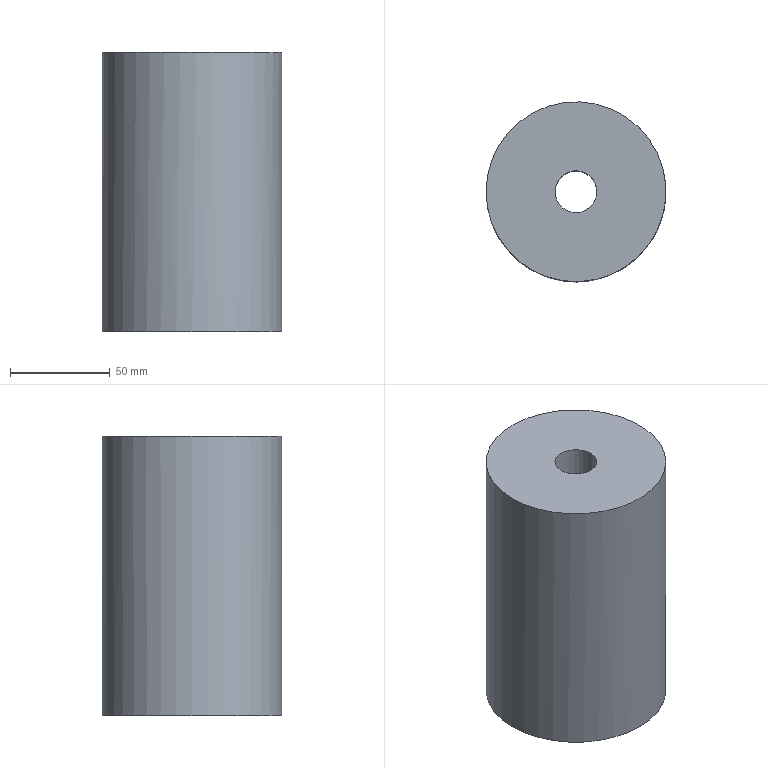Part | NX | features solid 2 | 1 solid | 4 faces | box 90 x 90 x 140 mm | volume 842151 mm3 | cylinder 2 | plane 2 | commonest cylinder face diameters 21 x1 90 x1
STEP:
#1=CARTESIAN_POINT('',(1440.,-535.,-125.));
#2=VERTEX_POINT('',#1);
#3=CARTESIAN_POINT('',(1395.,-535.,-125.));
#4=DIRECTION('',(0.,0.,-1.));
#5=DIRECTION('',(1.,0.,0.));
#6=AXIS2_PLACEMENT_3D('',#3,#4,#5);
#7=CIRCLE('',#6,45.);
#8=EDGE_CURVE('',#2,#2,#7,.F.);
#9=ORIENTED_EDGE('',*,*,#8,.T.);
#10=EDGE_LOOP('',(#9));
#11=FACE_BOUND('',#10,.T.);
#12=CARTESIAN_POINT('',(1350.,-535.,15.));
#13=VERTEX_POINT('',#12);
#14=CARTESIAN_POINT('',(1395.,-535.,15.));
#15=DIRECTION('',(0.,0.,1.));
#16=DIRECTION('',(-1.,0.,0.));
#17=AXIS2_PLACEMENT_3D('',#14,#15,#16);
#18=CIRCLE('',#17,45.);
#19=EDGE_CURVE('',#13,#13,#18,.T.);
#20=ORIENTED_EDGE('',*,*,#19,.F.);
#21=EDGE_LOOP('',(#20));
#22=FACE_BOUND('',#21,.T.);
#23=CARTESIAN_POINT('',(1395.,-535.,-125.));
#24=DIRECTION('',(0.,0.,-1.));
#25=DIRECTION('',(-0.9848,-0.1736,0.));
#26=AXIS2_PLACEMENT_3D('',#23,#24,#25);
#27=CYLINDRICAL_SURFACE('',#26,45.);
#28=ADVANCED_FACE('',(#11,#22),#27,.T.);
#29=CARTESIAN_POINT('',(1384.66,-536.823,-125.));
#30=VERTEX_POINT('',#29);
#31=CARTESIAN_POINT('',(1395.,-535.,-125.));
#32=DIRECTION('',(0.,0.,1.));
#33=DIRECTION('',(-0.9848,-0.1736,0.));
#34=AXIS2_PLACEMENT_3D('',#31,#32,#33);
#35=CIRCLE('',#34,10.5);
#36=EDGE_CURVE('',#30,#30,#35,.T.);
#37=ORIENTED_EDGE('',*,*,#36,.T.);
#38=EDGE_LOOP('',(#37));
#39=FACE_BOUND('',#38,.T.);
#40=ORIENTED_EDGE('',*,*,#8,.F.);
#41=EDGE_LOOP('',(#40));
#42=FACE_BOUND('',#41,.T.);
#43=CARTESIAN_POINT('',(1401.078,-569.468,-125.));
#44=DIRECTION('',(0.,0.,1.));
#45=DIRECTION('',(0.9848,0.1736,0.));
#46=AXIS2_PLACEMENT_3D('',#43,#44,#45);
#47=PLANE('',#46);
#48=ADVANCED_FACE('',(#39,#42),#47,.F.);
#49=CARTESIAN_POINT('',(1384.66,-536.823,15.));
#50=VERTEX_POINT('',#49);
#51=CARTESIAN_POINT('',(1395.,-535.,15.));
#52=DIRECTION('',(0.,0.,1.));
#53=DIRECTION('',(-0.9848,-0.1736,0.));
#54=AXIS2_PLACEMENT_3D('',#51,#52,#53);
#55=CIRCLE('',#54,10.5);
#56=EDGE_CURVE('',#50,#50,#55,.T.);
#57=ORIENTED_EDGE('',*,*,#56,.T.);
#58=EDGE_LOOP('',(#57));
#59=FACE_BOUND('',#58,.T.);
#60=ORIENTED_EDGE('',*,*,#36,.F.);
#61=EDGE_LOOP('',(#60));
#62=FACE_BOUND('',#61,.T.);
#63=CARTESIAN_POINT('',(1395.,-535.,-125.));
#64=DIRECTION('',(0.,0.,-1.));
#65=DIRECTION('',(-0.9848,-0.1736,0.));
#66=AXIS2_PLACEMENT_3D('',#63,#64,#65);
#67=CYLINDRICAL_SURFACE('',#66,10.5);
#68=ADVANCED_FACE('',(#59,#62),#67,.F.);
#69=ORIENTED_EDGE('',*,*,#19,.T.);
#70=EDGE_LOOP('',(#69));
#71=FACE_BOUND('',#70,.T.);
#72=ORIENTED_EDGE('',*,*,#56,.F.);
#73=EDGE_LOOP('',(#72));
#74=FACE_BOUND('',#73,.T.);
#75=CARTESIAN_POINT('',(1396.823,-545.34,15.));
#76=DIRECTION('',(0.,0.,-1.));
#77=DIRECTION('',(-0.9848,-0.1736,0.));
#78=AXIS2_PLACEMENT_3D('',#75,#76,#77);
#79=PLANE('',#78);
#80=ADVANCED_FACE('',(#71,#74),#79,.F.);
#81=CLOSED_SHELL('',(#28,#48,#68,#80));
#82=MANIFOLD_SOLID_BREP('',#81);
#83=(LENGTH_UNIT()NAMED_UNIT(*)SI_UNIT(.MILLI.,.METRE.));
#84=UNCERTAINTY_MEASURE_WITH_UNIT(LENGTH_MEASURE(0.00001),#83,'','');
#85=(NAMED_UNIT(*)PLANE_ANGLE_UNIT()SI_UNIT($,.RADIAN.));
#86=(NAMED_UNIT(*)SI_UNIT($,.STERADIAN.)SOLID_ANGLE_UNIT());
#87=(GEOMETRIC_REPRESENTATION_CONTEXT(3)GLOBAL_UNCERTAINTY_ASSIGNED_CONTEXT((#84))GLOBAL_UNIT_ASSIGNED_CONTEXT((#83,#85,#86))REPRESENTATION_CONTEXT('',''));
#88=ADVANCED_BREP_SHAPE_REPRESENTATION('',(#82),#87);